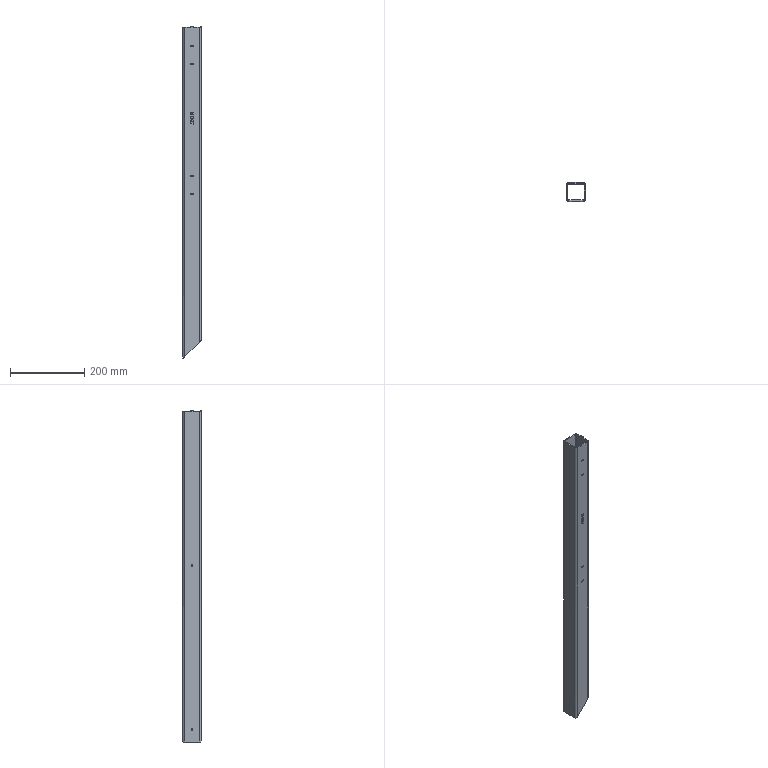Part | SolidWorks | features BaseBody 1 | 1 solid | 116 faces | box 50 x 50 x 893.5 mm | volume 467939 mm3 | plane 80 | spline 19 | cylinder 17 | commonest cylinder face diameters 4.2 x8 6 x4 12 x4 8 x1